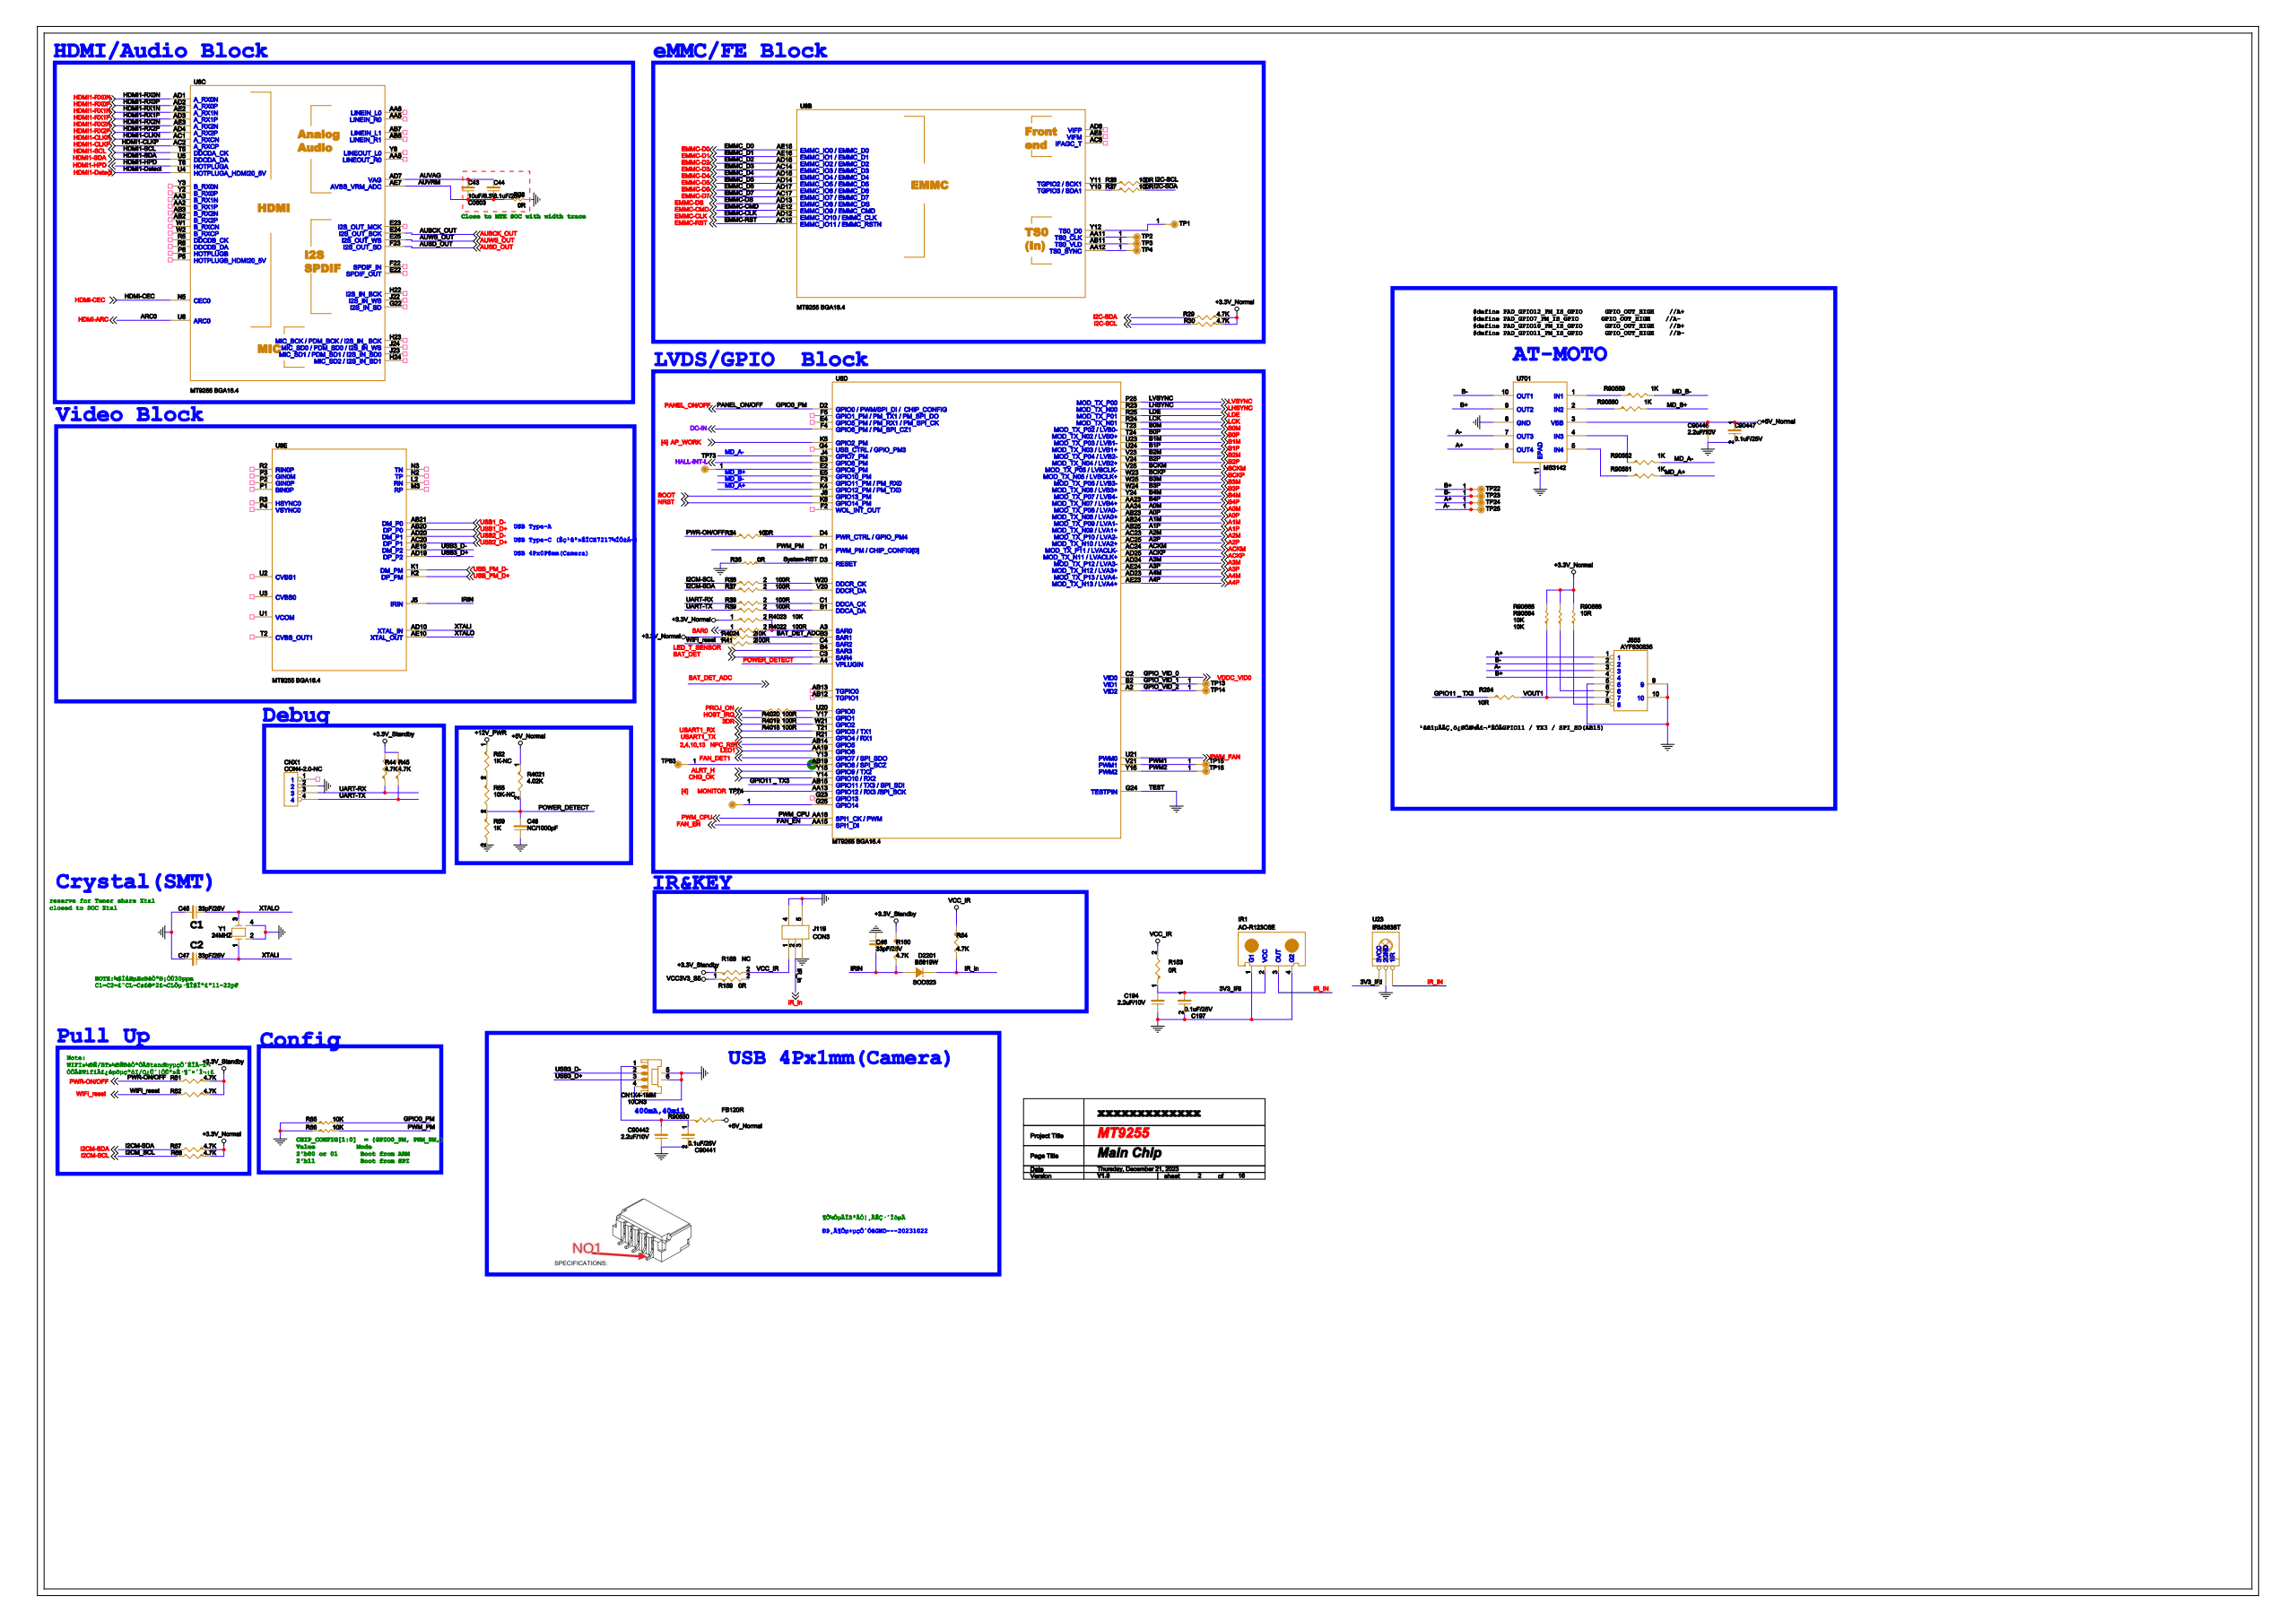Circuit board | Cadence Allegro | 1223 parts | 777 nets | one sheet of the schematic
Parts on this sheet (reference | value | footprint):
10CN3 | 4PIN-2.54-L-H-G | CN1X4-1MM
C43 | 10uF/6.3V | C0603
C44 | 0.1uF/25V | C0402
C45 | 33pF/25V | C0402
C46 | 33pF/25V | C0402
C47 | 33pF/25V | C0402
C48 | NC/1000pF | C0402
C194 | 2.2uF/10V | C0402
C197 | 0.1uF/25V | C0402
C90441 | 0.1uF/25V | C0402
C90442 | 2.2uF/10V | C0402
C90446 | 2.2uF/10V | C0402
C90447 | 0.1uF/25V | C0402
CNX1 | CON4-2.0-NC | DIP4PIN-2P0MM
D2201 | B5819W | SOD323
IR1 | AO-R123C6E | AO-R123C6E-HS
J119 | CON3 | CN1X3-0P8MM
J855 | AYF530835 | AYF530835
P2 | HDMI/90D | HDMI_A
R28 | 0R | R0402
R29 | 4.7K | R0402
R30 | 4.7K | R0402
R35 | 0R | R0402
R44 | 4.7K | R0402
R45 | 4.7K | R0402
R52 | 1K-NC | R0402
R54 | 4.7K | R0402
R55 | 10K-NC | R0402
R59 | 1K | R0402
R61 | 4.7K | R0402
R62 | 4.7K | R0402
R65 | 10K | R0402
R66 | 10K | R0402
R67 | 4.7K | R0402
R68 | 4.7K | R0402
R153 | 0R | R0402
R158 | NC | R0402
R159 | 0R | R0402
R160 | 4.7K | R0402
R264 | 10R | R0402
R4018 | 100R | R0402
R4019 | 100R | R0402
R4020 | 100R | R0402
R4021 | 4.02K | R0402
R4022 | 100R | R0402
R4023 | 10K | R0402
R90550 | FB120R | R0603
R90559 | 1K | R0402
R90560 | 1K | R0402
R90561 | 1K | R0402
R90562 | 1K | R0402
R90564 | 10K | R0402
R90565 | 10K | R0402
R90566 | 10R | R0402
TP1 | DEO | TP06MM
TP2 | DEO | TP06MM
TP3 | DEO | TP06MM
TP4 | DEO | TP06MM
TP13 | DEO | TP06MM
TP14 | DEO | TP06MM
TP15 | DEO | TP06MM
TP16 | DEO | TP06MM
TP22 | DEO | TP06MM
TP23 | DEO | TP06MM
TP24 | DEO | TP06MM
TP25 | DEO | TP06MM
TP73 | DEO | TP06MM
TP74 | DEO | TP06MM
TP83 | DEO | TP06MM
U8 | MT9255 BGA16.4 | LFBGA462
U23 | IRM3638T | IRM3638T
U701 | MS3142 | MS3142-MSOP10PP
Y1 | 24MHZ | CRY-D3225
Nets of these parts (net: part-pin ...):
GND: 10CN3-4 10CN3-5 10CN3-6 C45-1 C46-2 C47-1 C48-2 C194-2 C197-2 C90441-2 C90442-2 C90446-2 C90447-2 CNX1-2 IR1-1 IR1-4 J119-3 J119-4 J119-5 J855-5 J855-9 J855-10 R28-2 R35-2 R59-2 R65-1 R66-1 U23-2 U701-8 U701-11 Y1-2 Y1-4 P2-2 P2-5 P2-8 P2-11 P2-21 U8-G24
N25107431: 10CN3-1 C90441-1 C90442-1 R90550-1
USB3_D-: 10CN3-2 U8-AE19
USB3_D+: 10CN3-3 U8-AD19
I2C-SCL: R30-2
I2C-SDA: R29-2
MONITOR: U8-AA13
NPC_RST: U8-AB14
+12V_PWR: R52-1
+3.3V_STANDBY: R44-2 R45-2 R61-1 R62-1 R158-1 R160-1
+5V_NORMAL: C90446-1 C90447-1 R4021-1 R90550-2 U701-3
+3.3V_EMMC: R29-1 R30-1 R67-1 R68-1 R4023-1 R90564-2 R90565-2 R90566-2
VCC3V3_S5: R159-1
XTALO: C45-2 Y1-3 U8-AE10
IRIN: C46-1 D2201-1 R160-2 U8-J5
XTALI: C47-2 Y1-1 U8-AD10
3V3_IRI: C194-1 C197-1 IR1-2 R153-1 U23-3
AUVAG: C43-1 C44-1 U8-AD7
AUVRM: C43-2 C44-2 R28-1 U8-AE7
POWER_DETECT: C48-1 R55-2 R59-1 R4021-2 U8-A4
BAT_DET_ADC: U8-B3
HDMI-ARC: U8-U6
UART-RX: CNX1-3 R44-1
UART-TX: CNX1-4 R45-1
USART1_TX: U8-R21
USART1_RX: U8-T21
IR_IN: D2201-2 IR1-3 J119-2 R54-2 U23-1
N23354576: TP1-1 U8-Y12
GPIO_VID_1: TP13-1 U8-B2
GPIO_VID_2: TP14-1 U8-A2
PWM1: TP15-1 U8-V21
PWM2: TP16-1 U8-Y16
N23354579: TP2-1 U8-AA11
B+: J855-4 TP22-1 U701-9
B-: J855-2 TP23-1 U701-10
A+: J855-1 TP24-1 U701-6
A-: J855-3 TP25-1 U701-7
N23354577: TP3-1 U8-AB11
N23354578: TP4-1 U8-AA12
BAT_DET: U8-C3
N24969908: TP73-1 U8-E2
N24820965: TP74-1 U8-G25
N25970483: TP83-1 U8-AB19
HOST_IRQ: R4019-2
PROJ_ON: R4020-2
VCC_IR: J119-1 R54-1 R153-2 R158-2 R159-2
WIFI_RESET: R62-2
LED_T_SENSOR: U8-B4
N25165373: J855-6 R90565-1
VOUT1: J855-7 R264-2 R90564-1
N25167371: J855-8 R90566-1
HDMI-CEC: P2-13 U8-N5
HDMI1-CLKP: P2-10 U8-AC2
HDMI1-CLKN: U8-AC1
HDMI1-RX1N: P2-6 U8-AE2
HDMI1-RX0P: P2-7 U8-AD2
HDMI1-RX0N: P2-9 U8-AD1
HDMI1-RX1P: P2-4 U8-AD3
HDMI1-RX2P: P2-1 U8-AD4
HDMI1-RX2N: P2-3 U8-AE3
USB1_D+: U8-AB20
VID0_3DREF: R4018-2
LVSYNC: U8-P25
LHSYNC: U8-R23
LDE: U8-R25
LCK: U8-R24
B0M: U8-T23
B0P: U8-T24
B1M: U8-U23
B1P: U8-U24
I2CM-SDA: R67-2
I2CM-SCL: R68-2
B2M: U8-V23
B2P: U8-V24
BCKM: U8-V25
BCKP: U8-W23
B3P: U8-W24
B4M: U8-Y24
B4P: U8-AA23
A0M: U8-AA24
A0P: U8-AB23
A1M: U8-AB24
A1P: U8-AB25
A2M: U8-AC23
A2P: U8-AC25
ACKM: U8-AC24
ACKP: U8-AD25
A3P: U8-AE24
A4M: U8-AD23
A4P: U8-AE23
PWR-ON/OFF: R61-2
FAN_EN: U8-AA15
PANEL_ON/OFF: R65-2 U8-D2
DC-IN: U8-F4
BOOT: U8-J6
NRST: U8-K6
AP_WORK: U8-K5
N24501236: R4018-1 U8-W21
N24501261: R4019-1 U8-Y17
N24501297: R4020-1 U8-U20
CHG_OK: U8-Y14
FAN_DET1: U8-Y13
PWM_FAN: U8-U21
PWM_CPU: U8-AA16
SAR0: R4022-1
N24648131: R4022-2 R4023-2 U8-A3
GPIO11 _ TX3: R264-1 U8-AB15
SYSTEM-RST: R35-1 U8-D3
LED1: U8-AA19
ALRT_H: U8-Y15
HALL-INT-L: U8-E3
EMMC-CMD: U8-AE12
N233452980: R52-2 R55-1
PWM_PM: R66-2 U8-D1
EMMC-CLK: U8-AD12
EMMC-DS: U8-AD13
N25148089: R90559-1 U701-1
MD_B-: R90559-2 U8-F3
N25148125: R90560-1 U701-2
MD_B+: R90560-2 U8-E5
N25148184: R90561-1 U701-5
MD_A+: R90561-2 U8-K4
N25207710: R90562-1 U701-4
MD_A-: R90562-2 U8-J4
HDMI1-SCL: U8-T5
HDMI1-SDA: U8-U5
HDMI1-HPD: U8-T6
EMMC-D0: U8-AE15
EMMC-D1: U8-AE16
EMMC-D2: U8-AD16
EMMC-D3: U8-AC14
EMMC-D4: U8-AD15
EMMC-D5: U8-AD14
EMMC-D6: U8-AD17
EMMC-D7: U8-AC17
EMMC-RST: U8-AC12
AUBCK_OUT: U8-E24
AUSD_OUT: U8-F23
AUWS_OUT: U8-E25